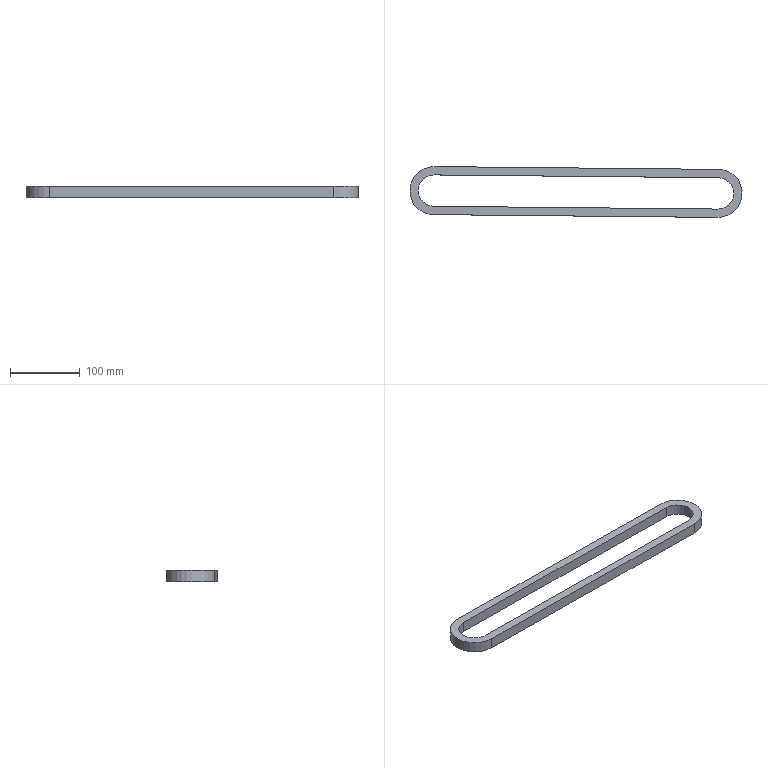Part | NX | features DATUM_CSYS 1, EXTRUDE 1, LINKED_FACE 1, SKETCH 1 | 1 solid | 10 faces | box 477.82 x 73.07 x 16 mm | volume 191391 mm3 | plane 6 | cylinder 4 | commonest cylinder face diameters 45.07 x2 69.07 x2
STEP:
#1=CARTESIAN_POINT('',(354.779,-59.327,16.));
#2=VERTEX_POINT('',#1);
#3=CARTESIAN_POINT('',(355.221,-14.259,16.));
#4=VERTEX_POINT('',#3);
#5=CARTESIAN_POINT('',(355.,-36.793,16.));
#6=DIRECTION('',(0.,0.,-1.));
#7=DIRECTION('',(-1.,0.,0.));
#8=AXIS2_PLACEMENT_3D('',#5,#6,#7);
#9=CIRCLE('',#8,22.535);
#10=EDGE_CURVE('',#2,#4,#9,.T.);
#11=ORIENTED_EDGE('',*,*,#10,.F.);
#12=CARTESIAN_POINT('',(354.779,-59.327,0.));
#13=VERTEX_POINT('',#12);
#14=CARTESIAN_POINT('',(354.779,-59.327,0.));
#15=DIRECTION('',(0.,0.,1.));
#16=VECTOR('',#15,1000.);
#17=LINE('',#14,#16);
#18=EDGE_CURVE('',#13,#2,#17,.T.);
#19=ORIENTED_EDGE('',*,*,#18,.F.);
#20=CARTESIAN_POINT('',(355.221,-14.259,0.));
#21=VERTEX_POINT('',#20);
#22=CARTESIAN_POINT('',(355.,-36.793,0.));
#23=DIRECTION('',(0.,0.,-1.));
#24=DIRECTION('',(-0.009785,-1.,0.));
#25=AXIS2_PLACEMENT_3D('',#22,#23,#24);
#26=CIRCLE('',#25,22.535);
#27=EDGE_CURVE('',#13,#21,#26,.T.);
#28=ORIENTED_EDGE('',*,*,#27,.T.);
#29=CARTESIAN_POINT('',(355.221,-14.259,0.));
#30=DIRECTION('',(0.,0.,1.));
#31=VECTOR('',#30,1000.);
#32=LINE('',#29,#31);
#33=EDGE_CURVE('',#21,#4,#32,.T.);
#34=ORIENTED_EDGE('',*,*,#33,.T.);
#35=EDGE_LOOP('',(#11,#19,#28,#34));
#36=FACE_BOUND('',#35,.T.);
#37=CARTESIAN_POINT('',(355.,-36.793,0.));
#38=DIRECTION('',(0.,0.,1.));
#39=DIRECTION('',(1.,0.,0.));
#40=AXIS2_PLACEMENT_3D('',#37,#38,#39);
#41=CYLINDRICAL_SURFACE('',#40,22.535);
#42=ADVANCED_FACE('',(#36),#41,.F.);
#43=CARTESIAN_POINT('',(763.971,-18.259,16.));
#44=VERTEX_POINT('',#43);
#45=CARTESIAN_POINT('',(355.221,-14.259,16.));
#46=DIRECTION('',(1.,-0.009785,0.));
#47=VECTOR('',#46,1000.);
#48=LINE('',#45,#47);
#49=EDGE_CURVE('',#4,#44,#48,.T.);
#50=ORIENTED_EDGE('',*,*,#49,.F.);
#51=ORIENTED_EDGE('',*,*,#33,.F.);
#52=CARTESIAN_POINT('',(763.971,-18.259,0.));
#53=VERTEX_POINT('',#52);
#54=CARTESIAN_POINT('',(355.221,-14.259,0.));
#55=DIRECTION('',(1.,-0.009785,0.));
#56=VECTOR('',#55,1000.);
#57=LINE('',#54,#56);
#58=EDGE_CURVE('',#21,#53,#57,.T.);
#59=ORIENTED_EDGE('',*,*,#58,.T.);
#60=CARTESIAN_POINT('',(763.971,-18.259,0.));
#61=DIRECTION('',(0.,0.,1.));
#62=VECTOR('',#61,1000.);
#63=LINE('',#60,#62);
#64=EDGE_CURVE('',#53,#44,#63,.T.);
#65=ORIENTED_EDGE('',*,*,#64,.T.);
#66=EDGE_LOOP('',(#50,#51,#59,#65));
#67=FACE_BOUND('',#66,.T.);
#68=CARTESIAN_POINT('',(355.221,-14.259,0.));
#69=DIRECTION('',(-0.009785,-1.,0.));
#70=DIRECTION('',(1.,-0.009785,0.));
#71=AXIS2_PLACEMENT_3D('',#68,#69,#70);
#72=PLANE('',#71);
#73=ADVANCED_FACE('',(#67),#72,.T.);
#74=CARTESIAN_POINT('',(763.529,-63.327,16.));
#75=VERTEX_POINT('',#74);
#76=CARTESIAN_POINT('',(763.75,-40.793,16.));
#77=DIRECTION('',(0.,0.,-1.));
#78=DIRECTION('',(0.009785,1.,0.));
#79=AXIS2_PLACEMENT_3D('',#76,#77,#78);
#80=CIRCLE('',#79,22.535);
#81=EDGE_CURVE('',#44,#75,#80,.T.);
#82=ORIENTED_EDGE('',*,*,#81,.F.);
#83=ORIENTED_EDGE('',*,*,#64,.F.);
#84=CARTESIAN_POINT('',(763.529,-63.327,0.));
#85=VERTEX_POINT('',#84);
#86=CARTESIAN_POINT('',(763.75,-40.793,0.));
#87=DIRECTION('',(0.,0.,-1.));
#88=DIRECTION('',(0.009785,1.,0.));
#89=AXIS2_PLACEMENT_3D('',#86,#87,#88);
#90=CIRCLE('',#89,22.535);
#91=EDGE_CURVE('',#53,#85,#90,.T.);
#92=ORIENTED_EDGE('',*,*,#91,.T.);
#93=CARTESIAN_POINT('',(763.529,-63.327,0.));
#94=DIRECTION('',(0.,0.,1.));
#95=VECTOR('',#94,1000.);
#96=LINE('',#93,#95);
#97=EDGE_CURVE('',#85,#75,#96,.T.);
#98=ORIENTED_EDGE('',*,*,#97,.T.);
#99=EDGE_LOOP('',(#82,#83,#92,#98));
#100=FACE_BOUND('',#99,.T.);
#101=CARTESIAN_POINT('',(763.75,-40.793,0.));
#102=DIRECTION('',(0.,0.,1.));
#103=DIRECTION('',(1.,0.,0.));
#104=AXIS2_PLACEMENT_3D('',#101,#102,#103);
#105=CYLINDRICAL_SURFACE('',#104,22.535);
#106=ADVANCED_FACE('',(#100),#105,.F.);
#107=CARTESIAN_POINT('',(354.662,-71.326,16.));
#108=VERTEX_POINT('',#107);
#109=CARTESIAN_POINT('',(763.412,-75.326,16.));
#110=VERTEX_POINT('',#109);
#111=CARTESIAN_POINT('',(354.662,-71.326,16.));
#112=DIRECTION('',(1.,-0.009785,0.));
#113=VECTOR('',#112,1000.);
#114=LINE('',#111,#113);
#115=EDGE_CURVE('',#108,#110,#114,.T.);
#116=ORIENTED_EDGE('',*,*,#115,.F.);
#117=CARTESIAN_POINT('',(354.662,-71.326,0.));
#118=VERTEX_POINT('',#117);
#119=CARTESIAN_POINT('',(354.662,-71.326,0.));
#120=DIRECTION('',(0.,0.,1.));
#121=VECTOR('',#120,1000.);
#122=LINE('',#119,#121);
#123=EDGE_CURVE('',#118,#108,#122,.T.);
#124=ORIENTED_EDGE('',*,*,#123,.F.);
#125=CARTESIAN_POINT('',(763.412,-75.326,0.));
#126=VERTEX_POINT('',#125);
#127=CARTESIAN_POINT('',(354.662,-71.326,0.));
#128=DIRECTION('',(1.,-0.009785,0.));
#129=VECTOR('',#128,1000.);
#130=LINE('',#127,#129);
#131=EDGE_CURVE('',#118,#126,#130,.T.);
#132=ORIENTED_EDGE('',*,*,#131,.T.);
#133=CARTESIAN_POINT('',(763.412,-75.326,0.));
#134=DIRECTION('',(0.,0.,1.));
#135=VECTOR('',#134,1000.);
#136=LINE('',#133,#135);
#137=EDGE_CURVE('',#126,#110,#136,.T.);
#138=ORIENTED_EDGE('',*,*,#137,.T.);
#139=EDGE_LOOP('',(#116,#124,#132,#138));
#140=FACE_BOUND('',#139,.T.);
#141=CARTESIAN_POINT('',(354.662,-71.326,0.));
#142=DIRECTION('',(-0.009785,-1.,0.));
#143=DIRECTION('',(1.,-0.009785,0.));
#144=AXIS2_PLACEMENT_3D('',#141,#142,#143);
#145=PLANE('',#144);
#146=ADVANCED_FACE('',(#140),#145,.T.);
#147=CARTESIAN_POINT('',(764.088,-6.26,16.));
#148=VERTEX_POINT('',#147);
#149=CARTESIAN_POINT('',(763.75,-40.793,16.));
#150=DIRECTION('',(0.,0.,1.));
#151=DIRECTION('',(-0.009785,-1.,0.));
#152=AXIS2_PLACEMENT_3D('',#149,#150,#151);
#153=CIRCLE('',#152,34.535);
#154=EDGE_CURVE('',#110,#148,#153,.T.);
#155=ORIENTED_EDGE('',*,*,#154,.F.);
#156=ORIENTED_EDGE('',*,*,#137,.F.);
#157=CARTESIAN_POINT('',(764.088,-6.26,0.));
#158=VERTEX_POINT('',#157);
#159=CARTESIAN_POINT('',(763.75,-40.793,0.));
#160=DIRECTION('',(0.,0.,1.));
#161=DIRECTION('',(-0.009785,-1.,0.));
#162=AXIS2_PLACEMENT_3D('',#159,#160,#161);
#163=CIRCLE('',#162,34.535);
#164=EDGE_CURVE('',#126,#158,#163,.T.);
#165=ORIENTED_EDGE('',*,*,#164,.T.);
#166=CARTESIAN_POINT('',(764.088,-6.26,0.));
#167=DIRECTION('',(0.,0.,1.));
#168=VECTOR('',#167,1000.);
#169=LINE('',#166,#168);
#170=EDGE_CURVE('',#158,#148,#169,.T.);
#171=ORIENTED_EDGE('',*,*,#170,.T.);
#172=EDGE_LOOP('',(#155,#156,#165,#171));
#173=FACE_BOUND('',#172,.T.);
#174=CARTESIAN_POINT('',(763.75,-40.793,0.));
#175=DIRECTION('',(0.,0.,1.));
#176=DIRECTION('',(1.,0.,0.));
#177=AXIS2_PLACEMENT_3D('',#174,#175,#176);
#178=CYLINDRICAL_SURFACE('',#177,34.535);
#179=ADVANCED_FACE('',(#173),#178,.T.);
#180=CARTESIAN_POINT('',(355.338,-2.26,16.));
#181=VERTEX_POINT('',#180);
#182=CARTESIAN_POINT('',(764.088,-6.26,16.));
#183=DIRECTION('',(-1.,0.009785,0.));
#184=VECTOR('',#183,1000.);
#185=LINE('',#182,#184);
#186=EDGE_CURVE('',#148,#181,#185,.T.);
#187=ORIENTED_EDGE('',*,*,#186,.F.);
#188=ORIENTED_EDGE('',*,*,#170,.F.);
#189=CARTESIAN_POINT('',(355.338,-2.26,0.));
#190=VERTEX_POINT('',#189);
#191=CARTESIAN_POINT('',(764.088,-6.26,0.));
#192=DIRECTION('',(-1.,0.009785,0.));
#193=VECTOR('',#192,1000.);
#194=LINE('',#191,#193);
#195=EDGE_CURVE('',#158,#190,#194,.T.);
#196=ORIENTED_EDGE('',*,*,#195,.T.);
#197=CARTESIAN_POINT('',(355.338,-2.26,0.));
#198=DIRECTION('',(0.,0.,1.));
#199=VECTOR('',#198,1000.);
#200=LINE('',#197,#199);
#201=EDGE_CURVE('',#190,#181,#200,.T.);
#202=ORIENTED_EDGE('',*,*,#201,.T.);
#203=EDGE_LOOP('',(#187,#188,#196,#202));
#204=FACE_BOUND('',#203,.T.);
#205=CARTESIAN_POINT('',(764.088,-6.26,0.));
#206=DIRECTION('',(0.009785,1.,0.));
#207=DIRECTION('',(-1.,0.009785,0.));
#208=AXIS2_PLACEMENT_3D('',#205,#206,#207);
#209=PLANE('',#208);
#210=ADVANCED_FACE('',(#204),#209,.T.);
#211=CARTESIAN_POINT('',(355.,-36.793,16.));
#212=DIRECTION('',(0.,0.,1.));
#213=DIRECTION('',(0.009785,1.,0.));
#214=AXIS2_PLACEMENT_3D('',#211,#212,#213);
#215=CIRCLE('',#214,34.535);
#216=EDGE_CURVE('',#181,#108,#215,.T.);
#217=ORIENTED_EDGE('',*,*,#216,.F.);
#218=ORIENTED_EDGE('',*,*,#201,.F.);
#219=CARTESIAN_POINT('',(355.,-36.793,0.));
#220=DIRECTION('',(0.,0.,1.));
#221=DIRECTION('',(-1.,0.,0.));
#222=AXIS2_PLACEMENT_3D('',#219,#220,#221);
#223=CIRCLE('',#222,34.535);
#224=EDGE_CURVE('',#190,#118,#223,.T.);
#225=ORIENTED_EDGE('',*,*,#224,.T.);
#226=ORIENTED_EDGE('',*,*,#123,.T.);
#227=EDGE_LOOP('',(#217,#218,#225,#226));
#228=FACE_BOUND('',#227,.T.);
#229=CARTESIAN_POINT('',(355.,-36.793,0.));
#230=DIRECTION('',(0.,0.,1.));
#231=DIRECTION('',(1.,0.,0.));
#232=AXIS2_PLACEMENT_3D('',#229,#230,#231);
#233=CYLINDRICAL_SURFACE('',#232,34.535);
#234=ADVANCED_FACE('',(#228),#233,.T.);
#235=CARTESIAN_POINT('',(763.529,-63.327,16.));
#236=DIRECTION('',(-1.,0.009785,0.));
#237=VECTOR('',#236,1000.);
#238=LINE('',#235,#237);
#239=EDGE_CURVE('',#75,#2,#238,.T.);
#240=ORIENTED_EDGE('',*,*,#239,.F.);
#241=ORIENTED_EDGE('',*,*,#97,.F.);
#242=CARTESIAN_POINT('',(763.529,-63.327,0.));
#243=DIRECTION('',(-1.,0.009785,0.));
#244=VECTOR('',#243,1000.);
#245=LINE('',#242,#244);
#246=EDGE_CURVE('',#85,#13,#245,.T.);
#247=ORIENTED_EDGE('',*,*,#246,.T.);
#248=ORIENTED_EDGE('',*,*,#18,.T.);
#249=EDGE_LOOP('',(#240,#241,#247,#248));
#250=FACE_BOUND('',#249,.T.);
#251=CARTESIAN_POINT('',(763.529,-63.327,0.));
#252=DIRECTION('',(0.009785,1.,0.));
#253=DIRECTION('',(-1.,0.009785,0.));
#254=AXIS2_PLACEMENT_3D('',#251,#252,#253);
#255=PLANE('',#254);
#256=ADVANCED_FACE('',(#250),#255,.T.);
#257=ORIENTED_EDGE('',*,*,#224,.F.);
#258=ORIENTED_EDGE('',*,*,#195,.F.);
#259=ORIENTED_EDGE('',*,*,#164,.F.);
#260=ORIENTED_EDGE('',*,*,#131,.F.);
#261=EDGE_LOOP('',(#257,#258,#259,#260));
#262=FACE_BOUND('',#261,.T.);
#263=ORIENTED_EDGE('',*,*,#27,.F.);
#264=ORIENTED_EDGE('',*,*,#246,.F.);
#265=ORIENTED_EDGE('',*,*,#91,.F.);
#266=ORIENTED_EDGE('',*,*,#58,.F.);
#267=EDGE_LOOP('',(#263,#264,#265,#266));
#268=FACE_BOUND('',#267,.T.);
#269=CARTESIAN_POINT('',(355.,-36.793,0.));
#270=DIRECTION('',(0.,0.,1.));
#271=DIRECTION('',(1.,0.,0.));
#272=AXIS2_PLACEMENT_3D('',#269,#270,#271);
#273=PLANE('',#272);
#274=ADVANCED_FACE('',(#262,#268),#273,.F.);
#275=ORIENTED_EDGE('',*,*,#216,.T.);
#276=ORIENTED_EDGE('',*,*,#115,.T.);
#277=ORIENTED_EDGE('',*,*,#154,.T.);
#278=ORIENTED_EDGE('',*,*,#186,.T.);
#279=EDGE_LOOP('',(#275,#276,#277,#278));
#280=FACE_BOUND('',#279,.T.);
#281=ORIENTED_EDGE('',*,*,#239,.T.);
#282=ORIENTED_EDGE('',*,*,#10,.T.);
#283=ORIENTED_EDGE('',*,*,#49,.T.);
#284=ORIENTED_EDGE('',*,*,#81,.T.);
#285=EDGE_LOOP('',(#281,#282,#283,#284));
#286=FACE_BOUND('',#285,.T.);
#287=CARTESIAN_POINT('',(355.,-36.793,16.));
#288=DIRECTION('',(0.,0.,1.));
#289=DIRECTION('',(1.,0.,0.));
#290=AXIS2_PLACEMENT_3D('',#287,#288,#289);
#291=PLANE('',#290);
#292=ADVANCED_FACE('',(#280,#286),#291,.T.);
#293=CLOSED_SHELL('',(#42,#73,#106,#146,#179,#210,#234,#256,#274,#292));
#294=MANIFOLD_SOLID_BREP('',#293);
#295=(LENGTH_UNIT()NAMED_UNIT(*)SI_UNIT(.MILLI.,.METRE.));
#296=UNCERTAINTY_MEASURE_WITH_UNIT(LENGTH_MEASURE(0.00001),#295,'','');
#297=(NAMED_UNIT(*)PLANE_ANGLE_UNIT()SI_UNIT($,.RADIAN.));
#298=(NAMED_UNIT(*)SI_UNIT($,.STERADIAN.)SOLID_ANGLE_UNIT());
#299=(GEOMETRIC_REPRESENTATION_CONTEXT(3)GLOBAL_UNCERTAINTY_ASSIGNED_CONTEXT((#296))GLOBAL_UNIT_ASSIGNED_CONTEXT((#295,#297,#298))REPRESENTATION_CONTEXT('',''));
#300=ADVANCED_BREP_SHAPE_REPRESENTATION('',(#294),#299);